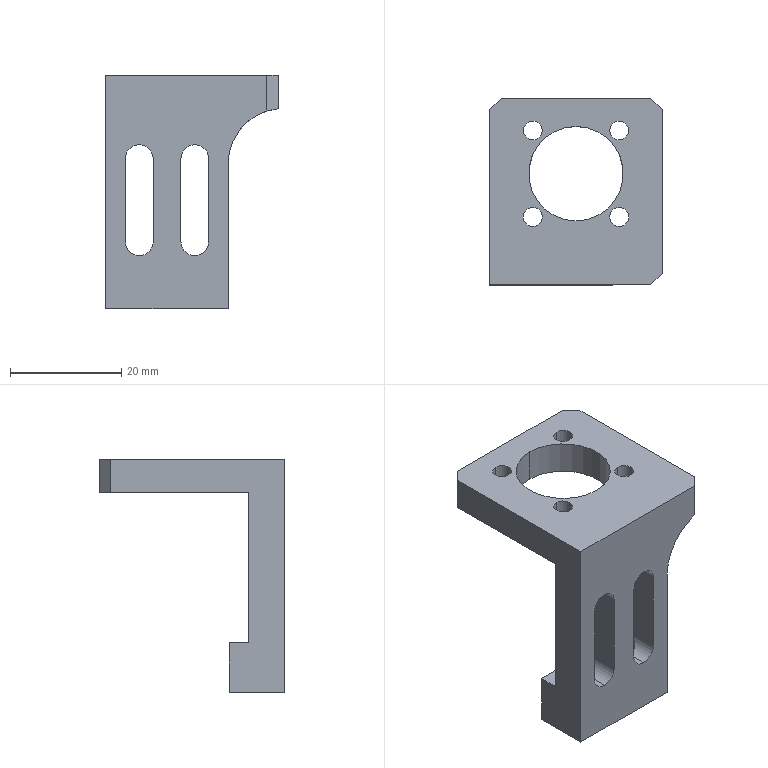NC program | NX | posted with a generic post | part box 31 x 33.478 x 42 mm
Lines 48 to 875 of 3423:
(ZLEVEL_PROFILE , TOOL : D10)
N82 T15 M6
N84 G54
N86 G17 G0 G90 X8.429 Y-21.839 B0. C0. S9500 M3
N88 G43 Z30. H15
N90 Z1.5
N92 G94 G1 X-16.054 Z0.217 F1000.
N94 X-17.398 Y-21.505 Z0.144
N96 X-18.604 Y-20.823 Z0.072
N98 X-19.584 Y-19.844 Z-0.001
N100 X-20.266 Y-18.638 Z-0.074
N102 X-20.6 Y-17.293 Z-0.146
N104 Y-1. Z-1.
N106 Y14.739 F3000.
N108 G2 X-19.106 Y18.345 R5.1
N110 G1 X-17.106 Y20.345
N112 G2 X-13.5 Y21.839 R5.1
N114 G1 X13.5
N116 G2 X17.106 Y20.345 R5.1
N118 G1 X19.106 Y18.345
N120 G2 X20.6 Y14.739 R5.1
N122 G1 Y-14.739
N124 G2 X19.106 Y-18.345 R5.1
N126 G1 X17.106 Y-20.345
N128 G2 X13.5 Y-21.839 R5.1
N130 G1 X-15.5
N132 G2 X-20.6 Y-16.739 R5.1
N134 G1 Y-1.
N136 Y14.739 Z-1.1
N138 X-20.575 Y15.239 Z-1.103
N140 X-20.502 Y15.734 Z-1.106
N142 X-20.38 Y16.22 Z-1.109
N144 X-20.212 Y16.691 Z-1.113
N146 X-19.998 Y17.143 Z-1.116
N148 X-19.74 Y17.572 Z-1.119
N150 X-19.442 Y17.974 Z-1.122
N152 X-19.106 Y18.345 Z-1.125
N154 X-17.106 Y20.345 Z-1.143
N156 X-16.735 Y20.681 Z-1.147
N158 X-16.333 Y20.98 Z-1.15
N160 X-15.904 Y21.237 Z-1.153
N162 X-15.452 Y21.451 Z-1.156
N164 X-14.98 Y21.619 Z-1.159
N166 X-14.495 Y21.741 Z-1.162
N168 X-14. Y21.815 Z-1.166
N170 X-13.5 Y21.839 Z-1.169
N172 X13.5 Z-1.34
N174 X14. Y21.815 Z-1.343
N176 X14.495 Y21.741 Z-1.347
N178 X14.98 Y21.619 Z-1.35
N180 X15.452 Y21.451 Z-1.353
N182 X15.904 Y21.237 Z-1.356
N184 X16.333 Y20.98 Z-1.359
N186 X16.735 Y20.681 Z-1.362
N188 X17.106 Y20.345 Z-1.366
N190 X19.106 Y18.345 Z-1.384
N192 X19.442 Y17.974 Z-1.387
N194 X19.74 Y17.572 Z-1.39
N196 X19.998 Y17.143 Z-1.393
N198 X20.212 Y16.691 Z-1.396
N200 X20.38 Y16.22 Z-1.399
N202 X20.502 Y15.734 Z-1.403
N204 X20.575 Y15.239 Z-1.406
N206 X20.6 Y14.739 Z-1.409
N208 Y-14.739 Z-1.596
N210 X20.575 Y-15.239 Z-1.599
N212 X20.502 Y-15.734 Z-1.603
N214 X20.38 Y-16.22 Z-1.606
N216 X20.212 Y-16.691 Z-1.609
N218 X19.998 Y-17.143 Z-1.612
N220 X19.74 Y-17.572 Z-1.615
N222 X19.442 Y-17.974 Z-1.618
N224 X19.106 Y-18.345 Z-1.622
N226 X17.106 Y-20.345 Z-1.64
N228 X16.735 Y-20.681 Z-1.643
N230 X16.333 Y-20.98 Z-1.646
N232 X15.904 Y-21.237 Z-1.649
N234 X15.452 Y-21.451 Z-1.652
N236 X14.98 Y-21.619 Z-1.655
N238 X14.495 Y-21.741 Z-1.659
N240 X14. Y-21.815 Z-1.662
N242 X13.5 Y-21.839 Z-1.665
N244 X-15.5 Z-1.849
N246 X-16. Y-21.815 Z-1.852
N248 X-16.495 Y-21.741 Z-1.856
N250 X-16.98 Y-21.619 Z-1.859
N252 X-17.452 Y-21.451 Z-1.862
N254 X-17.904 Y-21.237 Z-1.865
N256 X-18.333 Y-20.98 Z-1.868
N258 X-18.735 Y-20.681 Z-1.871
N260 X-19.106 Y-20.345 Z-1.875
N262 X-19.442 Y-19.974 Z-1.878
N264 X-19.74 Y-19.572 Z-1.881
N266 X-19.998 Y-19.143 Z-1.884
N268 X-20.212 Y-18.691 Z-1.887
N270 X-20.38 Y-18.22 Z-1.891
N272 X-20.502 Y-17.734 Z-1.894
N274 X-20.575 Y-17.239 Z-1.897
N276 X-20.6 Y-16.739 Z-1.9
N278 Y-1. Z-2.
N280 Y14.739 Z-2.1
N282 X-20.575 Y15.239 Z-2.103
N284 X-20.502 Y15.734 Z-2.106
N286 X-20.38 Y16.22 Z-2.109
N288 X-20.212 Y16.691 Z-2.113
N290 X-19.998 Y17.143 Z-2.116
N292 X-19.74 Y17.572 Z-2.119
N294 X-19.442 Y17.974 Z-2.122
N296 X-19.106 Y18.345 Z-2.125
N298 X-17.106 Y20.345 Z-2.143
N300 X-16.735 Y20.681 Z-2.147
N302 X-16.333 Y20.98 Z-2.15
N304 X-15.904 Y21.237 Z-2.153
N306 X-15.452 Y21.451 Z-2.156
N308 X-14.98 Y21.619 Z-2.159
N310 X-14.495 Y21.741 Z-2.162
N312 X-14. Y21.815 Z-2.166
N314 X-13.5 Y21.839 Z-2.169
N316 X13.5 Z-2.34
N318 X14. Y21.815 Z-2.343
N320 X14.495 Y21.741 Z-2.347
N322 X14.98 Y21.619 Z-2.35
N324 X15.452 Y21.451 Z-2.353
N326 X15.904 Y21.237 Z-2.356
N328 X16.333 Y20.98 Z-2.359
N330 X16.735 Y20.681 Z-2.362
N332 X17.106 Y20.345 Z-2.366
N334 X19.106 Y18.345 Z-2.384
N336 X19.442 Y17.974 Z-2.387
N338 X19.74 Y17.572 Z-2.39
N340 X19.998 Y17.143 Z-2.393
N342 X20.212 Y16.691 Z-2.396
N344 X20.38 Y16.22 Z-2.399
N346 X20.502 Y15.734 Z-2.403
N348 X20.575 Y15.239 Z-2.406
N350 X20.6 Y14.739 Z-2.409
N352 Y-14.739 Z-2.596
N354 X20.575 Y-15.239 Z-2.599
N356 X20.502 Y-15.734 Z-2.603
N358 X20.38 Y-16.22 Z-2.606
N360 X20.212 Y-16.691 Z-2.609
N362 X19.998 Y-17.143 Z-2.612
N364 X19.74 Y-17.572 Z-2.615
N366 X19.442 Y-17.974 Z-2.618
N368 X19.106 Y-18.345 Z-2.622
N370 X17.106 Y-20.345 Z-2.64
N372 X16.735 Y-20.681 Z-2.643
N374 X16.333 Y-20.98 Z-2.646
N376 X15.904 Y-21.237 Z-2.649
N378 X15.452 Y-21.451 Z-2.652
N380 X14.98 Y-21.619 Z-2.655
N382 X14.495 Y-21.741 Z-2.659
N384 X14. Y-21.815 Z-2.662
N386 X13.5 Y-21.839 Z-2.665
N388 X-15.5 Z-2.849
N390 X-16. Y-21.815 Z-2.852
N392 X-16.495 Y-21.741 Z-2.856
N394 X-16.98 Y-21.619 Z-2.859
N396 X-17.452 Y-21.451 Z-2.862
N398 X-17.904 Y-21.237 Z-2.865
N400 X-18.333 Y-20.98 Z-2.868
N402 X-18.735 Y-20.681 Z-2.871
N404 X-19.106 Y-20.345 Z-2.875
N406 X-19.442 Y-19.974 Z-2.878
N408 X-19.74 Y-19.572 Z-2.881
N410 X-19.998 Y-19.143 Z-2.884
N412 X-20.212 Y-18.691 Z-2.887
N414 X-20.38 Y-18.22 Z-2.891
N416 X-20.502 Y-17.734 Z-2.894
N418 X-20.575 Y-17.239 Z-2.897
N420 X-20.6 Y-16.739 Z-2.9
N422 Y-1. Z-3.
N424 Y14.739 Z-3.1
N426 X-20.575 Y15.239 Z-3.103
N428 X-20.502 Y15.734 Z-3.106
N430 X-20.38 Y16.22 Z-3.109
N432 X-20.212 Y16.691 Z-3.113
N434 X-19.998 Y17.143 Z-3.116
N436 X-19.74 Y17.572 Z-3.119
N438 X-19.442 Y17.974 Z-3.122
N440 X-19.106 Y18.345 Z-3.125
N442 X-17.106 Y20.345 Z-3.143
N444 X-16.735 Y20.681 Z-3.147
N446 X-16.333 Y20.98 Z-3.15
N448 X-15.904 Y21.237 Z-3.153
N450 X-15.452 Y21.451 Z-3.156
N452 X-14.98 Y21.619 Z-3.159
N454 X-14.495 Y21.741 Z-3.162
N456 X-14. Y21.815 Z-3.166
N458 X-13.5 Y21.839 Z-3.169
N460 X13.5 Z-3.34
N462 X14. Y21.815 Z-3.343
N464 X14.495 Y21.741 Z-3.347
N466 X14.98 Y21.619 Z-3.35
N468 X15.452 Y21.451 Z-3.353
N470 X15.904 Y21.237 Z-3.356
N472 X16.333 Y20.98 Z-3.359
N474 X16.735 Y20.681 Z-3.362
N476 X17.106 Y20.345 Z-3.366
N478 X19.106 Y18.345 Z-3.384
N480 X19.442 Y17.974 Z-3.387
N482 X19.74 Y17.572 Z-3.39
N484 X19.998 Y17.143 Z-3.393
N486 X20.212 Y16.691 Z-3.396
N488 X20.38 Y16.22 Z-3.399
N490 X20.502 Y15.734 Z-3.403
N492 X20.575 Y15.239 Z-3.406
N494 X20.6 Y14.739 Z-3.409
N496 Y-14.739 Z-3.596
N498 X20.575 Y-15.239 Z-3.599
N500 X20.502 Y-15.734 Z-3.603
N502 X20.38 Y-16.22 Z-3.606
N504 X20.212 Y-16.691 Z-3.609
N506 X19.998 Y-17.143 Z-3.612
N508 X19.74 Y-17.572 Z-3.615
N510 X19.442 Y-17.974 Z-3.618
N512 X19.106 Y-18.345 Z-3.622
N514 X17.106 Y-20.345 Z-3.64
N516 X16.735 Y-20.681 Z-3.643
N518 X16.333 Y-20.98 Z-3.646
N520 X15.904 Y-21.237 Z-3.649
N522 X15.452 Y-21.451 Z-3.652
N524 X14.98 Y-21.619 Z-3.655
N526 X14.495 Y-21.741 Z-3.659
N528 X14. Y-21.815 Z-3.662
N530 X13.5 Y-21.839 Z-3.665
N532 X-15.5 Z-3.849
N534 X-16. Y-21.815 Z-3.852
N536 X-16.495 Y-21.741 Z-3.856
N538 X-16.98 Y-21.619 Z-3.859
N540 X-17.452 Y-21.451 Z-3.862
N542 X-17.904 Y-21.237 Z-3.865
N544 X-18.333 Y-20.98 Z-3.868
N546 X-18.735 Y-20.681 Z-3.871
N548 X-19.106 Y-20.345 Z-3.875
N550 X-19.442 Y-19.974 Z-3.878
N552 X-19.74 Y-19.572 Z-3.881
N554 X-19.998 Y-19.143 Z-3.884
N556 X-20.212 Y-18.691 Z-3.887
N558 X-20.38 Y-18.22 Z-3.891
N560 X-20.502 Y-17.734 Z-3.894
N562 X-20.575 Y-17.239 Z-3.897
N564 X-20.6 Y-16.739 Z-3.9
N566 Y-1. Z-4.
N568 Y14.739 Z-4.1
N570 X-20.575 Y15.239 Z-4.103
N572 X-20.502 Y15.734 Z-4.106
N574 X-20.38 Y16.22 Z-4.109
N576 X-20.212 Y16.691 Z-4.113
N578 X-19.998 Y17.143 Z-4.116
N580 X-19.74 Y17.572 Z-4.119
N582 X-19.442 Y17.974 Z-4.122
N584 X-19.106 Y18.345 Z-4.125
N586 X-17.106 Y20.345 Z-4.143
N588 X-16.735 Y20.681 Z-4.147
N590 X-16.333 Y20.98 Z-4.15
N592 X-15.904 Y21.237 Z-4.153
N594 X-15.452 Y21.451 Z-4.156
N596 X-14.98 Y21.619 Z-4.159
N598 X-14.495 Y21.741 Z-4.162
N600 X-14. Y21.815 Z-4.166
N602 X-13.5 Y21.839 Z-4.169
N604 X13.5 Z-4.34
N606 X14. Y21.815 Z-4.343
N608 X14.495 Y21.741 Z-4.347
N610 X14.98 Y21.619 Z-4.35
N612 X15.452 Y21.451 Z-4.353
N614 X15.904 Y21.237 Z-4.356
N616 X16.333 Y20.98 Z-4.359
N618 X16.735 Y20.681 Z-4.362
N620 X17.106 Y20.345 Z-4.366
N622 X19.106 Y18.345 Z-4.384
N624 X19.442 Y17.974 Z-4.387
N626 X19.74 Y17.572 Z-4.39
N628 X19.998 Y17.143 Z-4.393
N630 X20.212 Y16.691 Z-4.396
N632 X20.38 Y16.22 Z-4.399
N634 X20.502 Y15.734 Z-4.403
N636 X20.575 Y15.239 Z-4.406
N638 X20.6 Y14.739 Z-4.409
N640 Y-14.739 Z-4.596
N642 X20.575 Y-15.239 Z-4.599
N644 X20.502 Y-15.734 Z-4.603
N646 X20.38 Y-16.22 Z-4.606
N648 X20.212 Y-16.691 Z-4.609
N650 X19.998 Y-17.143 Z-4.612
N652 X19.74 Y-17.572 Z-4.615
N654 X19.442 Y-17.974 Z-4.618
N656 X19.106 Y-18.345 Z-4.622
N658 X17.106 Y-20.345 Z-4.64
N660 X16.735 Y-20.681 Z-4.643
N662 X16.333 Y-20.98 Z-4.646
N664 X15.904 Y-21.237 Z-4.649
N666 X15.452 Y-21.451 Z-4.652
N668 X14.98 Y-21.619 Z-4.655
N670 X14.495 Y-21.741 Z-4.659
N672 X14. Y-21.815 Z-4.662
N674 X13.5 Y-21.839 Z-4.665
N676 X-15.5 Z-4.849
N678 X-16. Y-21.815 Z-4.852
N680 X-16.495 Y-21.741 Z-4.856
N682 X-16.98 Y-21.619 Z-4.859
N684 X-17.452 Y-21.451 Z-4.862
N686 X-17.904 Y-21.237 Z-4.865
N688 X-18.333 Y-20.98 Z-4.868
N690 X-18.735 Y-20.681 Z-4.871
N692 X-19.106 Y-20.345 Z-4.875
N694 X-19.442 Y-19.974 Z-4.878
N696 X-19.74 Y-19.572 Z-4.881
N698 X-19.998 Y-19.143 Z-4.884
N700 X-20.212 Y-18.691 Z-4.887
N702 X-20.38 Y-18.22 Z-4.891
N704 X-20.502 Y-17.734 Z-4.894
N706 X-20.575 Y-17.239 Z-4.897
N708 X-20.6 Y-16.739 Z-4.9
N710 Y-1. Z-5.
N712 Y14.739 Z-5.1
N714 X-20.575 Y15.239 Z-5.103
N716 X-20.502 Y15.734 Z-5.106
N718 X-20.38 Y16.22 Z-5.109
N720 X-20.212 Y16.691 Z-5.113
N722 X-19.998 Y17.143 Z-5.116
N724 X-19.74 Y17.572 Z-5.119
N726 X-19.442 Y17.974 Z-5.122
N728 X-19.106 Y18.345 Z-5.125
N730 X-17.106 Y20.345 Z-5.143
N732 X-16.735 Y20.681 Z-5.147
N734 X-16.333 Y20.98 Z-5.15
N736 X-15.904 Y21.237 Z-5.153
N738 X-15.452 Y21.451 Z-5.156
N740 X-14.98 Y21.619 Z-5.159
N742 X-14.495 Y21.741 Z-5.162
N744 X-14. Y21.815 Z-5.166
N746 X-13.5 Y21.839 Z-5.169
N748 X13.5 Z-5.34
N750 X14. Y21.815 Z-5.343
N752 X14.495 Y21.741 Z-5.347
N754 X14.98 Y21.619 Z-5.35
N756 X15.452 Y21.451 Z-5.353
N758 X15.904 Y21.237 Z-5.356
N760 X16.333 Y20.98 Z-5.359
N762 X16.735 Y20.681 Z-5.362
N764 X17.106 Y20.345 Z-5.366
N766 X19.106 Y18.345 Z-5.384
N768 X19.442 Y17.974 Z-5.387
N770 X19.74 Y17.572 Z-5.39
N772 X19.998 Y17.143 Z-5.393
N774 X20.212 Y16.691 Z-5.396
N776 X20.38 Y16.22 Z-5.399
N778 X20.502 Y15.734 Z-5.403
N780 X20.575 Y15.239 Z-5.406
N782 X20.6 Y14.739 Z-5.409
N784 Y-14.739 Z-5.596
N786 X20.575 Y-15.239 Z-5.599
N788 X20.502 Y-15.734 Z-5.603
N790 X20.38 Y-16.22 Z-5.606
N792 X20.212 Y-16.691 Z-5.609
N794 X19.998 Y-17.143 Z-5.612
N796 X19.74 Y-17.572 Z-5.615
N798 X19.442 Y-17.974 Z-5.618
N800 X19.106 Y-18.345 Z-5.622
N802 X17.106 Y-20.345 Z-5.64
N804 X16.735 Y-20.681 Z-5.643
N806 X16.333 Y-20.98 Z-5.646
N808 X15.904 Y-21.237 Z-5.649
N810 X15.452 Y-21.451 Z-5.652
N812 X14.98 Y-21.619 Z-5.655
N814 X14.495 Y-21.741 Z-5.659
N816 X14. Y-21.815 Z-5.662
N818 X13.5 Y-21.839 Z-5.665
N820 X-15.5 Z-5.849
N822 X-16. Y-21.815 Z-5.852
N824 X-16.495 Y-21.741 Z-5.856
N826 X-16.98 Y-21.619 Z-5.859
N828 X-17.452 Y-21.451 Z-5.862
N830 X-17.904 Y-21.237 Z-5.865
N832 X-18.333 Y-20.98 Z-5.868
N834 X-18.735 Y-20.681 Z-5.871
N836 X-19.106 Y-20.345 Z-5.875
N838 X-19.442 Y-19.974 Z-5.878
N840 X-19.74 Y-19.572 Z-5.881
N842 X-19.998 Y-19.143 Z-5.884
N844 X-20.212 Y-18.691 Z-5.887
N846 X-20.38 Y-18.22 Z-5.891
N848 X-20.502 Y-17.734 Z-5.894
N850 X-20.575 Y-17.239 Z-5.897
N852 X-20.6 Y-16.739 Z-5.9
N854 Y-1. Z-6.
N856 Y14.739 Z-6.1
N858 X-20.575 Y15.239 Z-6.103
N860 X-20.502 Y15.734 Z-6.106
N862 X-20.38 Y16.22 Z-6.109
N864 X-20.212 Y16.691 Z-6.113
N866 X-19.998 Y17.143 Z-6.116
N868 X-19.74 Y17.572 Z-6.119
N870 X-19.442 Y17.974 Z-6.122
N872 X-19.106 Y18.345 Z-6.125
N874 X-17.106 Y20.345 Z-6.143
N876 X-16.735 Y20.681 Z-6.147
N878 X-16.333 Y20.98 Z-6.15
N880 X-15.904 Y21.237 Z-6.153
N882 X-15.452 Y21.451 Z-6.156
N884 X-14.98 Y21.619 Z-6.159
N886 X-14.495 Y21.741 Z-6.162
N888 X-14. Y21.815 Z-6.166
N890 X-13.5 Y21.839 Z-6.169
N892 X13.5 Z-6.34
N894 X14. Y21.815 Z-6.343
N896 X14.495 Y21.741 Z-6.347
N898 X14.98 Y21.619 Z-6.35
N900 X15.452 Y21.451 Z-6.353
N902 X15.904 Y21.237 Z-6.356
N904 X16.333 Y20.98 Z-6.359
N906 X16.735 Y20.681 Z-6.362
N908 X17.106 Y20.345 Z-6.366
N910 X19.106 Y18.345 Z-6.384
N912 X19.442 Y17.974 Z-6.387
N914 X19.74 Y17.572 Z-6.39
N916 X19.998 Y17.143 Z-6.393
N918 X20.212 Y16.691 Z-6.396
N920 X20.38 Y16.22 Z-6.399
N922 X20.502 Y15.734 Z-6.403
N924 X20.575 Y15.239 Z-6.406
N926 X20.6 Y14.739 Z-6.409
N928 Y-14.739 Z-6.596
N930 X20.575 Y-15.239 Z-6.599
N932 X20.502 Y-15.734 Z-6.603
N934 X20.38 Y-16.22 Z-6.606
N936 X20.212 Y-16.691 Z-6.609
N938 X19.998 Y-17.143 Z-6.612
N940 X19.74 Y-17.572 Z-6.615
N942 X19.442 Y-17.974 Z-6.618
N944 X19.106 Y-18.345 Z-6.622
N946 X17.106 Y-20.345 Z-6.64
N948 X16.735 Y-20.681 Z-6.643
N950 X16.333 Y-20.98 Z-6.646
N952 X15.904 Y-21.237 Z-6.649
N954 X15.452 Y-21.451 Z-6.652
N956 X14.98 Y-21.619 Z-6.655
N958 X14.495 Y-21.741 Z-6.659
N960 X14. Y-21.815 Z-6.662
N962 X13.5 Y-21.839 Z-6.665
N964 X-15.5 Z-6.849
N966 X-16. Y-21.815 Z-6.852
N968 X-16.495 Y-21.741 Z-6.856
N970 X-16.98 Y-21.619 Z-6.859
N972 X-17.452 Y-21.451 Z-6.862
N974 X-17.904 Y-21.237 Z-6.865
N976 X-18.333 Y-20.98 Z-6.868
N978 X-18.735 Y-20.681 Z-6.871
N980 X-19.106 Y-20.345 Z-6.875
N982 X-19.442 Y-19.974 Z-6.878
N984 X-19.74 Y-19.572 Z-6.881
N986 X-19.998 Y-19.143 Z-6.884
N988 X-20.212 Y-18.691 Z-6.887
N990 X-20.38 Y-18.22 Z-6.891
N992 X-20.502 Y-17.734 Z-6.894
N994 X-20.575 Y-17.239 Z-6.897
N996 X-20.6 Y-16.739 Z-6.9
N998 Y-1. Z-7.
N1000 Y14.739 Z-7.1
N1002 X-20.575 Y15.239 Z-7.103
N1004 X-20.502 Y15.734 Z-7.106
N1006 X-20.38 Y16.22 Z-7.109
N1008 X-20.212 Y16.691 Z-7.113
N1010 X-19.998 Y17.143 Z-7.116
N1012 X-19.74 Y17.572 Z-7.119
N1014 X-19.442 Y17.974 Z-7.122
N1016 X-19.106 Y18.345 Z-7.125
N1018 X-17.106 Y20.345 Z-7.143
N1020 X-16.735 Y20.681 Z-7.147
N1022 X-16.333 Y20.98 Z-7.15
N1024 X-15.904 Y21.237 Z-7.153
N1026 X-15.452 Y21.451 Z-7.156
N1028 X-14.98 Y21.619 Z-7.159
N1030 X-14.495 Y21.741 Z-7.162
N1032 X-14. Y21.815 Z-7.166
N1034 X-13.5 Y21.839 Z-7.169
N1036 X13.5 Z-7.34
N1038 X14. Y21.815 Z-7.343
N1040 X14.495 Y21.741 Z-7.347
N1042 X14.98 Y21.619 Z-7.35
N1044 X15.452 Y21.451 Z-7.353
N1046 X15.904 Y21.237 Z-7.356
N1048 X16.333 Y20.98 Z-7.359
N1050 X16.735 Y20.681 Z-7.362
N1052 X17.106 Y20.345 Z-7.366
N1054 X19.106 Y18.345 Z-7.384
N1056 X19.442 Y17.974 Z-7.387
N1058 X19.74 Y17.572 Z-7.39
N1060 X19.998 Y17.143 Z-7.393
N1062 X20.212 Y16.691 Z-7.396
N1064 X20.38 Y16.22 Z-7.399
N1066 X20.502 Y15.734 Z-7.403
N1068 X20.575 Y15.239 Z-7.406
N1070 X20.6 Y14.739 Z-7.409
N1072 Y-14.739 Z-7.596
N1074 X20.575 Y-15.239 Z-7.599
N1076 X20.502 Y-15.734 Z-7.603
N1078 X20.38 Y-16.22 Z-7.606
N1080 X20.212 Y-16.691 Z-7.609
N1082 X19.998 Y-17.143 Z-7.612
N1084 X19.74 Y-17.572 Z-7.615
N1086 X19.442 Y-17.974 Z-7.618
N1088 X19.106 Y-18.345 Z-7.622
N1090 X17.106 Y-20.345 Z-7.64
N1092 X16.735 Y-20.681 Z-7.643
N1094 X16.333 Y-20.98 Z-7.646
N1096 X15.904 Y-21.237 Z-7.649
N1098 X15.452 Y-21.451 Z-7.652
N1100 X14.98 Y-21.619 Z-7.655
N1102 X14.495 Y-21.741 Z-7.659
N1104 X14. Y-21.815 Z-7.662
N1106 X13.5 Y-21.839 Z-7.665
N1108 X-15.5 Z-7.849
N1110 X-16. Y-21.815 Z-7.852
N1112 X-16.495 Y-21.741 Z-7.856
N1114 X-16.98 Y-21.619 Z-7.859
N1116 X-17.452 Y-21.451 Z-7.862
N1118 X-17.904 Y-21.237 Z-7.865
N1120 X-18.333 Y-20.98 Z-7.868
N1122 X-18.735 Y-20.681 Z-7.871
N1124 X-19.106 Y-20.345 Z-7.875
N1126 X-19.442 Y-19.974 Z-7.878
N1128 X-19.74 Y-19.572 Z-7.881
N1130 X-19.998 Y-19.143 Z-7.884
N1132 X-20.212 Y-18.691 Z-7.887
N1134 X-20.38 Y-18.22 Z-7.891
N1136 X-20.502 Y-17.734 Z-7.894
N1138 X-20.575 Y-17.239 Z-7.897
N1140 X-20.6 Y-16.739 Z-7.9
N1142 Y-1. Z-8.
N1144 Y14.739 Z-8.1
N1146 X-20.575 Y15.239 Z-8.103
N1148 X-20.502 Y15.734 Z-8.106
N1150 X-20.38 Y16.22 Z-8.109
N1152 X-20.212 Y16.691 Z-8.113
N1154 X-19.998 Y17.143 Z-8.116
N1156 X-19.74 Y17.572 Z-8.119
N1158 X-19.442 Y17.974 Z-8.122
N1160 X-19.106 Y18.345 Z-8.125
N1162 X-17.106 Y20.345 Z-8.143
N1164 X-16.735 Y20.681 Z-8.147
N1166 X-16.333 Y20.98 Z-8.15
N1168 X-15.904 Y21.237 Z-8.153
N1170 X-15.452 Y21.451 Z-8.156
N1172 X-14.98 Y21.619 Z-8.159
N1174 X-14.495 Y21.741 Z-8.162
N1176 X-14. Y21.815 Z-8.166
N1178 X-13.5 Y21.839 Z-8.169
N1180 X13.5 Z-8.34
N1182 X14. Y21.815 Z-8.343
N1184 X14.495 Y21.741 Z-8.347
N1186 X14.98 Y21.619 Z-8.35
N1188 X15.452 Y21.451 Z-8.353
N1190 X15.904 Y21.237 Z-8.356
N1192 X16.333 Y20.98 Z-8.359
N1194 X16.735 Y20.681 Z-8.362
N1196 X17.106 Y20.345 Z-8.366
N1198 X19.106 Y18.345 Z-8.384
N1200 X19.442 Y17.974 Z-8.387
N1202 X19.74 Y17.572 Z-8.39
N1204 X19.998 Y17.143 Z-8.393
N1206 X20.212 Y16.691 Z-8.396
N1208 X20.38 Y16.22 Z-8.399
N1210 X20.502 Y15.734 Z-8.403
N1212 X20.575 Y15.239 Z-8.406
N1214 X20.6 Y14.739 Z-8.409
N1216 Y-14.739 Z-8.596
N1218 X20.575 Y-15.239 Z-8.599
N1220 X20.502 Y-15.734 Z-8.603
N1222 X20.38 Y-16.22 Z-8.606
N1224 X20.212 Y-16.691 Z-8.609
N1226 X19.998 Y-17.143 Z-8.612
N1228 X19.74 Y-17.572 Z-8.615
N1230 X19.442 Y-17.974 Z-8.618
N1232 X19.106 Y-18.345 Z-8.622
N1234 X17.106 Y-20.345 Z-8.64
N1236 X16.735 Y-20.681 Z-8.643
N1238 X16.333 Y-20.98 Z-8.646
N1240 X15.904 Y-21.237 Z-8.649
N1242 X15.452 Y-21.451 Z-8.652
N1244 X14.98 Y-21.619 Z-8.655
N1246 X14.495 Y-21.741 Z-8.659
N1248 X14. Y-21.815 Z-8.662
N1250 X13.5 Y-21.839 Z-8.665
N1252 X-15.5 Z-8.849
N1254 X-16. Y-21.815 Z-8.852
N1256 X-16.495 Y-21.741 Z-8.856
N1258 X-16.98 Y-21.619 Z-8.859
N1260 X-17.452 Y-21.451 Z-8.862
N1262 X-17.904 Y-21.237 Z-8.865
N1264 X-18.333 Y-20.98 Z-8.868
N1266 X-18.735 Y-20.681 Z-8.871
N1268 X-19.106 Y-20.345 Z-8.875
N1270 X-19.442 Y-19.974 Z-8.878
N1272 X-19.74 Y-19.572 Z-8.881
N1274 X-19.998 Y-19.143 Z-8.884
N1276 X-20.212 Y-18.691 Z-8.887
N1278 X-20.38 Y-18.22 Z-8.891
N1280 X-20.502 Y-17.734 Z-8.894
N1282 X-20.575 Y-17.239 Z-8.897
N1284 X-20.6 Y-16.739 Z-8.9
N1286 Y-1. Z-9.
N1288 Y14.739 Z-9.1
N1290 X-20.575 Y15.239 Z-9.103
N1292 X-20.502 Y15.734 Z-9.106
N1294 X-20.38 Y16.22 Z-9.109
N1296 X-20.212 Y16.691 Z-9.113
N1298 X-19.998 Y17.143 Z-9.116
N1300 X-19.74 Y17.572 Z-9.119
N1302 X-19.442 Y17.974 Z-9.122
N1304 X-19.106 Y18.345 Z-9.125
N1306 X-17.106 Y20.345 Z-9.143
N1308 X-16.735 Y20.681 Z-9.147
N1310 X-16.333 Y20.98 Z-9.15
N1312 X-15.904 Y21.237 Z-9.153
N1314 X-15.452 Y21.451 Z-9.156
N1316 X-14.98 Y21.619 Z-9.159
N1318 X-14.495 Y21.741 Z-9.162
N1320 X-14. Y21.815 Z-9.166
N1322 X-13.5 Y21.839 Z-9.169
N1324 X13.5 Z-9.34
N1326 X14. Y21.815 Z-9.343
N1328 X14.495 Y21.741 Z-9.347
N1330 X14.98 Y21.619 Z-9.35
N1332 X15.452 Y21.451 Z-9.353
N1334 X15.904 Y21.237 Z-9.356
N1336 X16.333 Y20.98 Z-9.359
N1338 X16.735 Y20.681 Z-9.362
N1340 X17.106 Y20.345 Z-9.366
N1342 X19.106 Y18.345 Z-9.384
N1344 X19.442 Y17.974 Z-9.387
N1346 X19.74 Y17.572 Z-9.39
N1348 X19.998 Y17.143 Z-9.393
N1350 X20.212 Y16.691 Z-9.396
N1352 X20.38 Y16.22 Z-9.399
N1354 X20.502 Y15.734 Z-9.403
N1356 X20.575 Y15.239 Z-9.406
N1358 X20.6 Y14.739 Z-9.409
N1360 Y-14.739 Z-9.596
N1362 X20.575 Y-15.239 Z-9.599
N1364 X20.502 Y-15.734 Z-9.603
N1366 X20.38 Y-16.22 Z-9.606
N1368 X20.212 Y-16.691 Z-9.609
N1370 X19.998 Y-17.143 Z-9.612
N1372 X19.74 Y-17.572 Z-9.615
N1374 X19.442 Y-17.974 Z-9.618
N1376 X19.106 Y-18.345 Z-9.622
N1378 X17.106 Y-20.345 Z-9.64
N1380 X16.735 Y-20.681 Z-9.643
N1382 X16.333 Y-20.98 Z-9.646
N1384 X15.904 Y-21.237 Z-9.649
N1386 X15.452 Y-21.451 Z-9.652
N1388 X14.98 Y-21.619 Z-9.655
N1390 X14.495 Y-21.741 Z-9.659
N1392 X14. Y-21.815 Z-9.662
N1394 X13.5 Y-21.839 Z-9.665
N1396 X-15.5 Z-9.849
N1398 X-16. Y-21.815 Z-9.852
N1400 X-16.495 Y-21.741 Z-9.856
N1402 X-16.98 Y-21.619 Z-9.859
N1404 X-17.452 Y-21.451 Z-9.862
N1406 X-17.904 Y-21.237 Z-9.865
N1408 X-18.333 Y-20.98 Z-9.868
N1410 X-18.735 Y-20.681 Z-9.871
N1412 X-19.106 Y-20.345 Z-9.875
N1414 X-19.442 Y-19.974 Z-9.878
N1416 X-19.74 Y-19.572 Z-9.881
N1418 X-19.998 Y-19.143 Z-9.884
N1420 X-20.212 Y-18.691 Z-9.887
N1422 X-20.38 Y-18.22 Z-9.891
N1424 X-20.502 Y-17.734 Z-9.894
N1426 X-20.575 Y-17.239 Z-9.897
N1428 X-20.6 Y-16.739 Z-9.9
N1430 Y-1. Z-10.
N1432 Y14.739 Z-10.1
N1434 X-20.575 Y15.239 Z-10.103
N1436 X-20.502 Y15.734 Z-10.106
N1438 X-20.38 Y16.22 Z-10.109
N1440 X-20.212 Y16.691 Z-10.113
N1442 X-19.998 Y17.143 Z-10.116
N1444 X-19.74 Y17.572 Z-10.119
N1446 X-19.442 Y17.974 Z-10.122
N1448 X-19.106 Y18.345 Z-10.125
N1450 X-17.106 Y20.345 Z-10.143
N1452 X-16.735 Y20.681 Z-10.147
N1454 X-16.333 Y20.98 Z-10.15
N1456 X-15.904 Y21.237 Z-10.153
N1458 X-15.452 Y21.451 Z-10.156
N1460 X-14.98 Y21.619 Z-10.159
N1462 X-14.495 Y21.741 Z-10.162
N1464 X-14. Y21.815 Z-10.166
N1466 X-13.5 Y21.839 Z-10.169
N1468 X13.5 Z-10.34
N1470 X14. Y21.815 Z-10.343
N1472 X14.495 Y21.741 Z-10.347
N1474 X14.98 Y21.619 Z-10.35
N1476 X15.452 Y21.451 Z-10.353
N1478 X15.904 Y21.237 Z-10.356
N1480 X16.333 Y20.98 Z-10.359
N1482 X16.735 Y20.681 Z-10.362
N1484 X17.106 Y20.345 Z-10.366
N1486 X19.106 Y18.345 Z-10.384
N1488 X19.442 Y17.974 Z-10.387
N1490 X19.74 Y17.572 Z-10.39
N1492 X19.998 Y17.143 Z-10.393
N1494 X20.212 Y16.691 Z-10.396
N1496 X20.38 Y16.22 Z-10.399
N1498 X20.502 Y15.734 Z-10.403
N1500 X20.575 Y15.239 Z-10.406
N1502 X20.6 Y14.739 Z-10.409
N1504 Y-14.739 Z-10.596
N1506 X20.575 Y-15.239 Z-10.599
N1508 X20.502 Y-15.734 Z-10.603
N1510 X20.38 Y-16.22 Z-10.606
N1512 X20.212 Y-16.691 Z-10.609
N1514 X19.998 Y-17.143 Z-10.612
N1516 X19.74 Y-17.572 Z-10.615
N1518 X19.442 Y-17.974 Z-10.618
N1520 X19.106 Y-18.345 Z-10.622
N1522 X17.106 Y-20.345 Z-10.64
N1524 X16.735 Y-20.681 Z-10.643
N1526 X16.333 Y-20.98 Z-10.646
N1528 X15.904 Y-21.237 Z-10.649
N1530 X15.452 Y-21.451 Z-10.652
N1532 X14.98 Y-21.619 Z-10.655
N1534 X14.495 Y-21.741 Z-10.659
N1536 X14. Y-21.815 Z-10.662
N1538 X13.5 Y-21.839 Z-10.665
N1540 X-15.5 Z-10.849
N1542 X-16. Y-21.815 Z-10.852
N1544 X-16.495 Y-21.741 Z-10.856
N1546 X-16.98 Y-21.619 Z-10.859
N1548 X-17.452 Y-21.451 Z-10.862
N1550 X-17.904 Y-21.237 Z-10.865
N1552 X-18.333 Y-20.98 Z-10.868
N1554 X-18.735 Y-20.681 Z-10.871
N1556 X-19.106 Y-20.345 Z-10.875
N1558 X-19.442 Y-19.974 Z-10.878
N1560 X-19.74 Y-19.572 Z-10.881
N1562 X-19.998 Y-19.143 Z-10.884
N1564 X-20.212 Y-18.691 Z-10.887
N1566 X-20.38 Y-18.22 Z-10.891
N1568 X-20.502 Y-17.734 Z-10.894
N1570 X-20.575 Y-17.239 Z-10.897
N1572 X-20.6 Y-16.739 Z-10.9
N1574 Y-1. Z-11.
N1576 Y14.739 Z-11.1
N1578 X-20.575 Y15.239 Z-11.103
N1580 X-20.502 Y15.734 Z-11.106
N1582 X-20.38 Y16.22 Z-11.109
N1584 X-20.212 Y16.691 Z-11.113
N1586 X-19.998 Y17.143 Z-11.116
N1588 X-19.74 Y17.572 Z-11.119
N1590 X-19.442 Y17.974 Z-11.122
N1592 X-19.106 Y18.345 Z-11.125
N1594 X-17.106 Y20.345 Z-11.143
N1596 X-16.735 Y20.681 Z-11.147
N1598 X-16.333 Y20.98 Z-11.15
N1600 X-15.904 Y21.237 Z-11.153
N1602 X-15.452 Y21.451 Z-11.156
N1604 X-14.98 Y21.619 Z-11.159
N1606 X-14.495 Y21.741 Z-11.162
N1608 X-14. Y21.815 Z-11.166
N1610 X-13.5 Y21.839 Z-11.169
N1612 X13.5 Z-11.34
N1614 X14. Y21.815 Z-11.343
N1616 X14.495 Y21.741 Z-11.347
N1618 X14.98 Y21.619 Z-11.35
N1620 X15.452 Y21.451 Z-11.353
N1622 X15.904 Y21.237 Z-11.356
N1624 X16.333 Y20.98 Z-11.359
N1626 X16.735 Y20.681 Z-11.362
N1628 X17.106 Y20.345 Z-11.366
N1630 X19.106 Y18.345 Z-11.384
N1632 X19.442 Y17.974 Z-11.387
N1634 X19.74 Y17.572 Z-11.39
N1636 X19.998 Y17.143 Z-11.393
N1638 X20.212 Y16.691 Z-11.396
N1640 X20.38 Y16.22 Z-11.399
N1642 X20.502 Y15.734 Z-11.403
N1644 X20.575 Y15.239 Z-11.406
N1646 X20.6 Y14.739 Z-11.409
N1648 Y-14.739 Z-11.596
N1650 X20.575 Y-15.239 Z-11.599
N1652 X20.502 Y-15.734 Z-11.603
N1654 X20.38 Y-16.22 Z-11.606
N1656 X20.212 Y-16.691 Z-11.609
N1658 X19.998 Y-17.143 Z-11.612
N1660 X19.74 Y-17.572 Z-11.615
N1662 X19.442 Y-17.974 Z-11.618
N1664 X19.106 Y-18.345 Z-11.622
N1666 X17.106 Y-20.345 Z-11.64
N1668 X16.735 Y-20.681 Z-11.643
N1670 X16.333 Y-20.98 Z-11.646
N1672 X15.904 Y-21.237 Z-11.649
N1674 X15.452 Y-21.451 Z-11.652
N1676 X14.98 Y-21.619 Z-11.655
N1678 X14.495 Y-21.741 Z-11.659
N1680 X14. Y-21.815 Z-11.662
N1682 X13.5 Y-21.839 Z-11.665
N1684 X-15.5 Z-11.849
N1686 X-16. Y-21.815 Z-11.852
N1688 X-16.495 Y-21.741 Z-11.856
N1690 X-16.98 Y-21.619 Z-11.859
N1692 X-17.452 Y-21.451 Z-11.862
N1694 X-17.904 Y-21.237 Z-11.865
N1696 X-18.333 Y-20.98 Z-11.868
N1698 X-18.735 Y-20.681 Z-11.871
N1700 X-19.106 Y-20.345 Z-11.875
N1702 X-19.442 Y-19.974 Z-11.878
N1704 X-19.74 Y-19.572 Z-11.881
N1706 X-19.998 Y-19.143 Z-11.884
N1708 X-20.212 Y-18.691 Z-11.887
N1710 X-20.38 Y-18.22 Z-11.891
N1712 X-20.502 Y-17.734 Z-11.894
N1714 X-20.575 Y-17.239 Z-11.897
N1716 X-20.6 Y-16.739 Z-11.9
N1718 Y-1. Z-12.
N1720 Y14.739 Z-12.1
N1722 X-20.575 Y15.239 Z-12.103
N1724 X-20.502 Y15.734 Z-12.106
N1726 X-20.38 Y16.22 Z-12.109
N1728 X-20.212 Y16.691 Z-12.113
N1730 X-19.998 Y17.143 Z-12.116